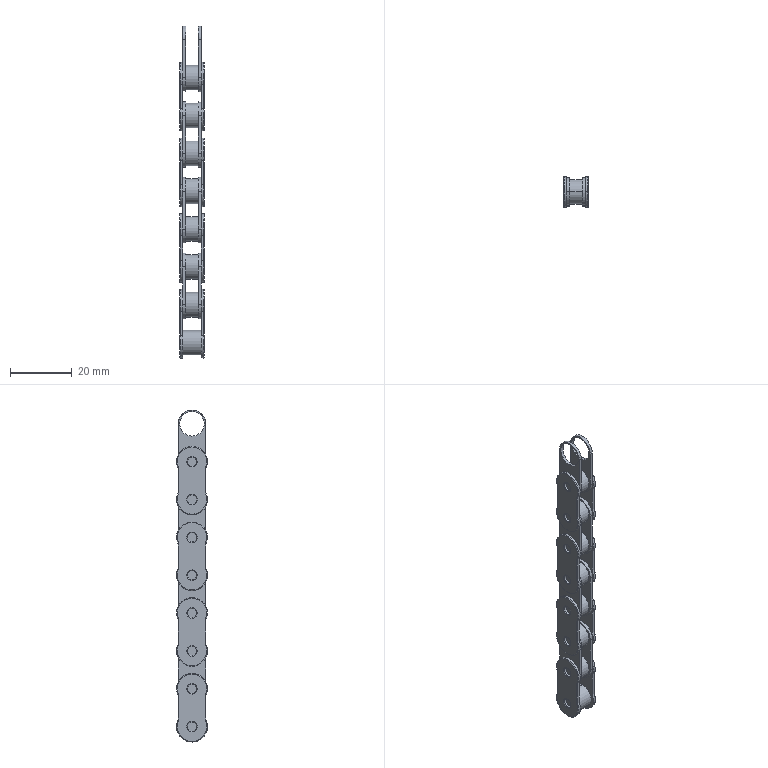Part | STEP file | 4 Chain Links v2 | 4 solids | 264 faces | box 8 x 10 x 107.9 mm | volume 4422 mm3 | cylinder 128 | plane 80 | torus 56 | commonest cylinder face diameters 3 x32 8 x32 9 x24 10 x24 0.4 x16